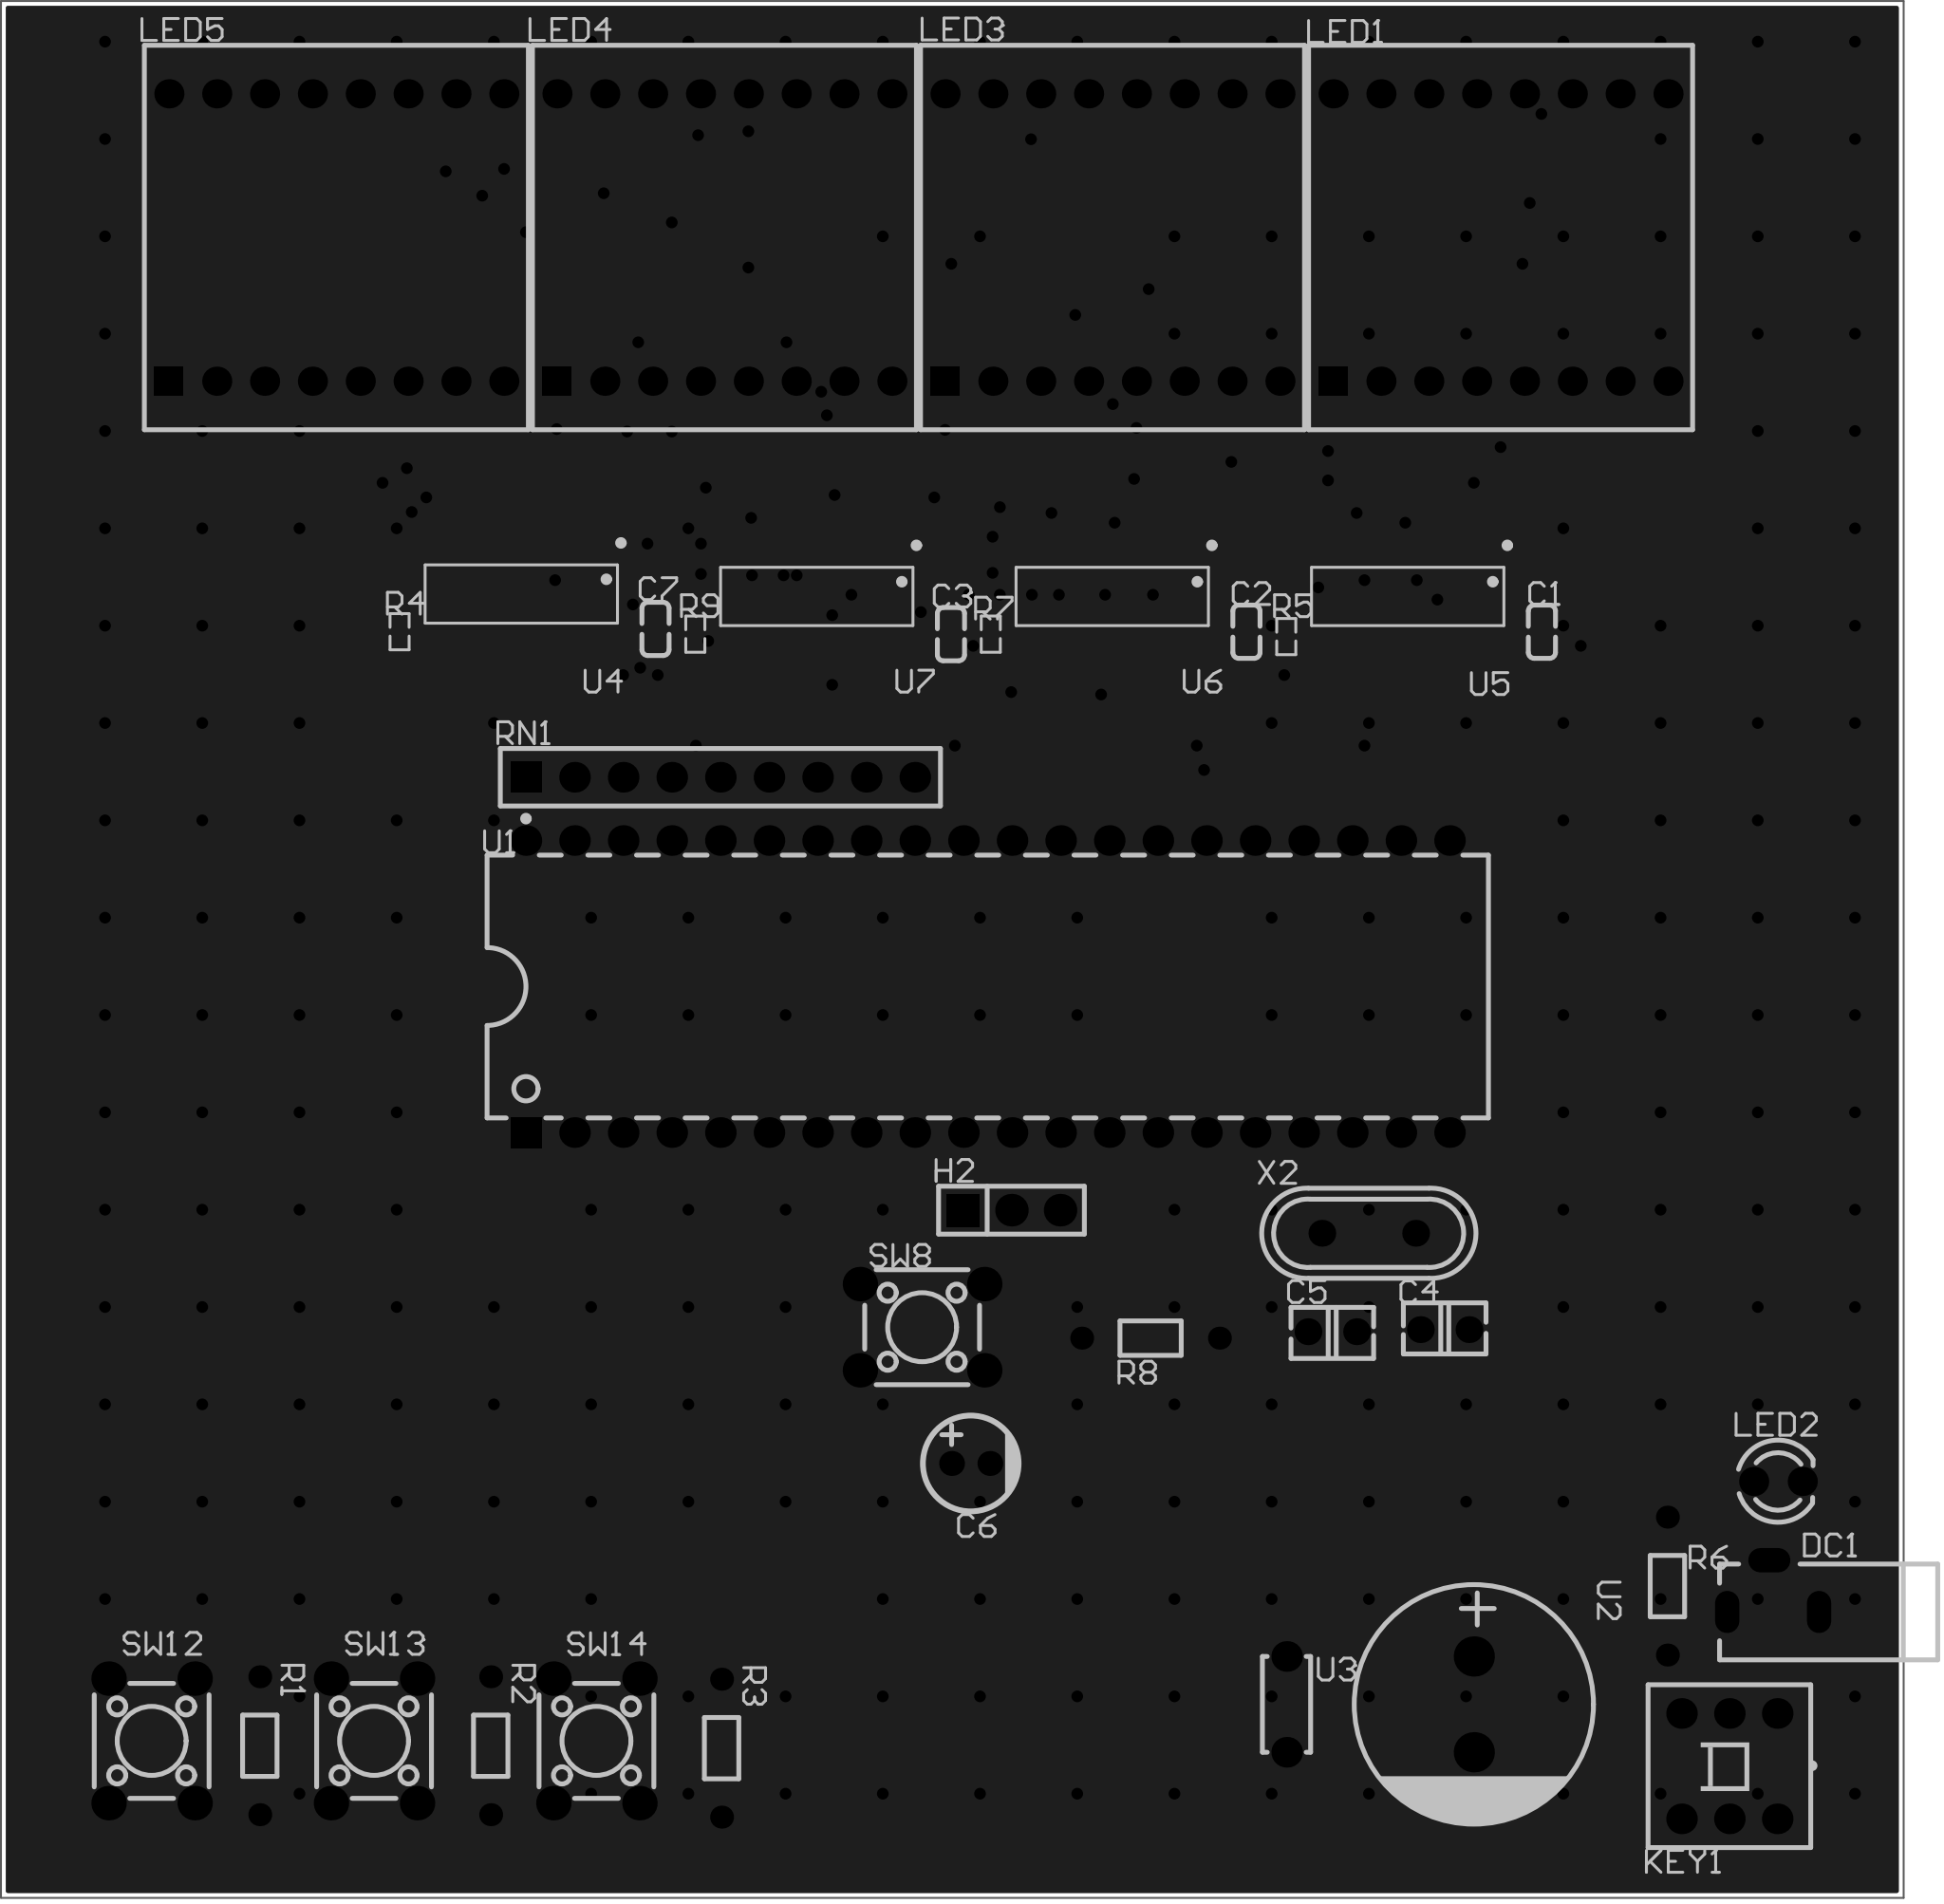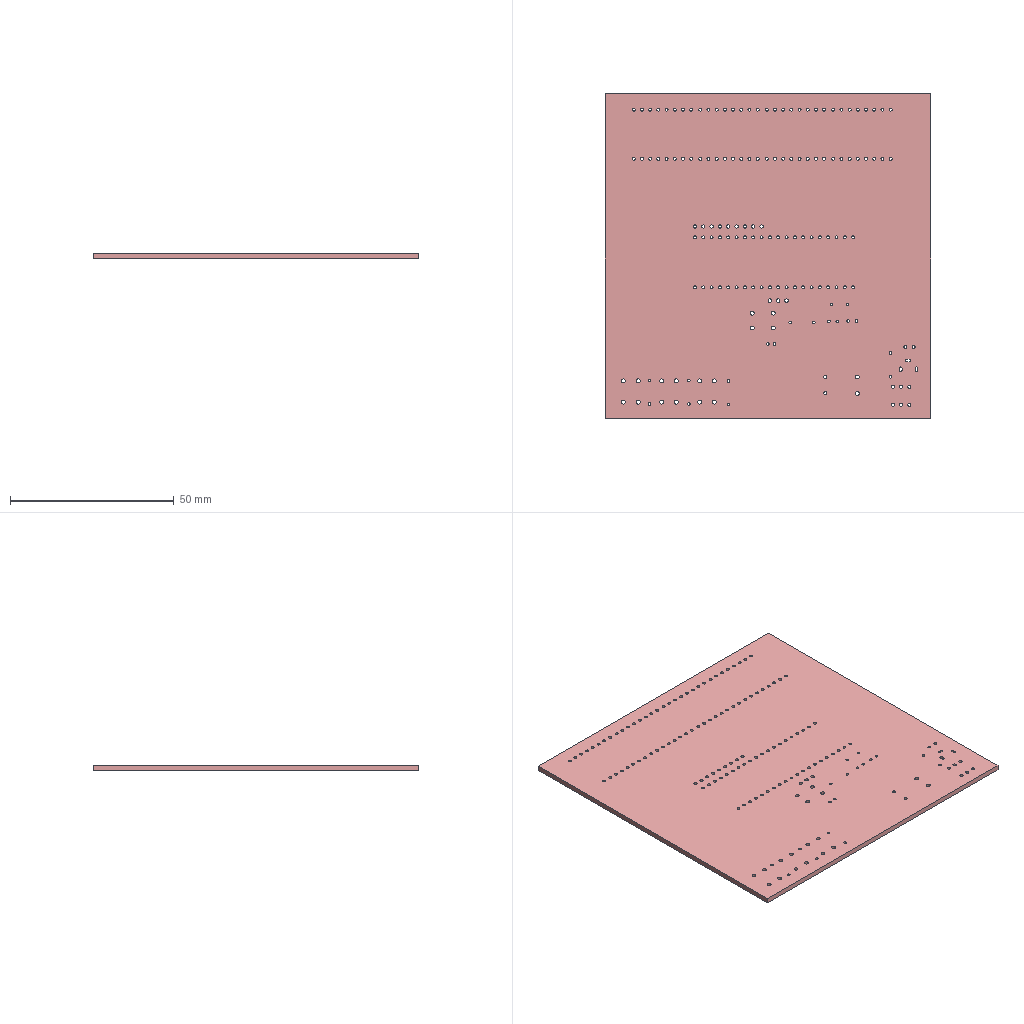Circuit board layout | Altium Designer | box 99.4 x 99 x 1.6 mm
Layer stack:
# Altium Designer layer stack of  (unit mm; dielectric type: 0 none, 1 core, 2 prepreg, 3 surface material)
index,name,kind,layer,copper_thickness_mm,dielectric_type,dielectric_thickness_mm,dielectric_material,dielectric_constant
0,Top Paste Mask Layer,other,,,,,,
1,Top Silkscreen Layer,other,,,,,,
2,Top Solder Mask Layer,dielectric,,,3,0.01,,3.3
3,Top Layer,copper,Top Layer,0.035,,,,
4,Dielectric1,dielectric,,,3,1.51,FR4,4.5
5,Bottom Layer,copper,Bottom Layer,0.035,,,,
6,Bottom Solder Mask Layer,dielectric,,,3,0.01,,3.3
7,Bottom Silkscreen Layer,other,,,,,,
8,Bottom Paste Mask Layer,other,,,,,,
# drill layer pairs: low layer,high layer
drill_pair,Top Layer,Bottom Layer
Part placement:
Designator,Comment,Layer,Footprint,Center-X(mm),Center-Y(mm),Rotation
C4,22pF,TopLayer,CAP-TH_L3.8-W2.5-P2.54-D0.50,157.988,115.57,180
C5,22pF,TopLayer,CAP-TH_L3.8-W2.5-P2.54-D0.50,152.116,115.461,0
C6,10uF,TopLayer,CAP-TH_BD5.0-P2.00-D0.8-FD-10UF50VC110GL,133.223,108.585,0
H2,,TopLayer,HDR-TH_3P-P2.54-V-M,135.352,121.805,0
KEY1,Non-latching switch 8.5×8.5 silent,TopLayer,SW-TH_6P-L8.5-W8.5-P2.54,172.865,92.787,180
LED2,,TopLayer,LED_TH-3mm,175.405,107.646,0
R8,10kΩ,TopLayer,Res_1/8W,142.621,115.126,180
R6,1kΩ,TopLayer,Res_1/8W,169.626,102.185,270
SW8,,TopLayer,SW-TH_4P-L6.0-W6.0-P4.50-LS6.5,130.683,115.697,0
SW12,,TopLayer,SW-TH_4P-L6.0-W6.0-P4.50-LS6.5,90.424,94.107,270
SW13,,TopLayer,SW-TH_4P-L6.0-W6.0-P4.50-LS6.5,102.044,94.107,270
SW14,,TopLayer,SW-TH_4P-L6.0-W6.0-P4.50-LS6.5,113.665,94.107,270
U1,STC89C52RC-40I-PDIP40,TopLayer,DIP-40_L52.0-W13.7-P2.54-LS15.2-BL,134.112,133.477,0
X2,11.059MHz,TopLayer,OSC-TH_L11.1-W4.7-P4.88,154.021,120.6,0
DC1,DC-002,TopLayer,DC-IN-TH_DC-3510,175.151,102.185,0
R1,10kΩ,TopLayer,Res_1/8W,96.075,93.853,270
R2,10kΩ,TopLayer,Res_1/8W,108.14,93.853,270
R3,10kΩ,TopLayer,Res_1/8W,120.205,93.726,270
RN1,-,TopLayer,RES-ARRAY-TH_9P-P2.54-D1.0,120.142,144.399,0
U2,1000uF,TopLayer,CAP-TH_BD12.5-P5.00-D0.6-FD,159.512,96.012,270
U3,100nF,TopLayer,CAP-TH_L5.0-W2.5-P5.00-D1.0,149.733,96.012,270
C1,100nF,TopLayer,C0603,163.068,151.995,270
C2,100nF,TopLayer,C0603,147.629,151.995,270
C3,100nF,TopLayer,C0603,132.19,151.868,270
C7,100nF,TopLayer,C0603,116.751,152.141,270
R4,10kΩ,TopLayer,R0402,103.378,151.995,270
R5,10kΩ,TopLayer,R0402,149.709,151.741,270
R7,10kΩ,TopLayer,R0402,134.27,151.868,270
R9,10kΩ,TopLayer,R0402,118.831,151.868,270
U4,74HC595D,118,TopLayer,SOIC-16_L9.9-W3.9-P1.27-LS6.0-BL,109.738,153.962,180
U5,74HC595D,118,TopLayer,SOIC-16_L9.9-W3.9-P1.27-LS6.0-BL,156.055,153.835,180
U6,74HC595D,118,TopLayer,SOIC-16_L9.9-W3.9-P1.27-LS6.0-BL,140.616,153.835,180
U7,74HC595D,118,TopLayer,SOIC-16_L9.9-W3.9-P1.27-LS6.0-BL,125.177,153.835,180
LED3,SLD0888FR1C1BD-3.5D,TopLayer,LED-MAT-TH_SLD0888FR1C1BD-3.5D,140.631,172.569,0
LED4,SLD0888FR1C1BD-3.5D,TopLayer,LED-MAT-TH_SLD0888FR1C1BD-3.5D,120.354,172.569,0
LED1,SLD0888FR1C1BD-3.5D,TopLayer,LED-MAT-TH_SLD0888FR1C1BD-3.5D,160.909,172.569,0
LED5,SLD0888FR1C1BD-3.5D,TopLayer,LED-MAT-TH_SLD0888FR1C1BD-3.5D,100.076,172.569,0
Pad and via stacks:
# Altium Designer via and pad stacks of  (unit mm). Each distinct definition once, with the count of objects using it.
# via: kind,start_layer,end_layer,hole_mm,diameter_mm,mode(0 simple;1 top-mid-bottom;2 full stack),diameter_per_layer,count,example_net
# pad: kind,layer,hole_mm,hole_type(0 round;1 square;2 slot),plating,top_size,top_shape(1 round;2 rect;3 octagon;9 rounded rect),mid_size,bottom_size,mode,footprint,size_per_layer,count,example
pad,Multi-Layer,0.8,0,plated,1.4x1.4,1,1.4x1.4,1.4x1.4,0,CAP-TH_L3.8-W2.5-P2.54-D0.50,,4,C4.1
pad,Multi-Layer,0.8,0,plated,1.3x1.3,1,1.3x1.3,1.3x1.3,0,CAP-TH_BD5.0-P2.00-D0.8-FD-10UF50VC110GL,,2,C6.2
pad,Multi-Layer,1.1,0,plated,1.7x1.7,2,1.7x1.7,1.7x1.7,0,HDR-TH_3P-P2.54-V-M,,1,H2.1
pad,Multi-Layer,1.1,0,plated,1.7x1.7,1,1.7x1.7,1.7x1.7,0,HDR-TH_3P-P2.54-V-M,,2,H2.2
pad,Multi-Layer,1,0,plated,1.6x1.6,1,1.6x1.6,1.6x1.6,0,SW-TH_6P-L8.5-W8.5-P2.54,,6,KEY1.4
pad,Multi-Layer,0.9144,0,plated,1.524x1.524,1,1.524x1.524,1.524x1.524,0,LED_TH-3mm,,2,LED2.1
pad,Multi-Layer,0.8001,0,plated,1.199x1.199,1,1.199x1.199,1.199x1.199,0,Res_1/8W,,10,R8.1
pad,Multi-Layer,1.2,0,plated,1.8x1.8,1,1.8x1.8,1.8x1.8,0,SW-TH_4P-L6.0-W6.0-P4.50-LS6.5,,16,SW8.1
pad,Multi-Layer,0.889,0,plated,1.6x1.6,1,1.6x1.6,1.6x1.6,0,DIP-40_L52.0-W13.7-P2.54-LS15.2-BL,,39,U1.31
pad,Multi-Layer,0.889,0,plated,1.6x1.6,2,1.6x1.6,1.6x1.6,0,DIP-40_L52.0-W13.7-P2.54-LS15.2-BL,,1,U1.1
pad,Multi-Layer,0.7,0,plated,1.4x1.4,1,1.4x1.4,1.4x1.4,0,OSC-TH_L11.1-W4.7-P4.88,,2,X2.1
pad,Multi-Layer,0.8,2,plated,2.2x1.27,1,2.2x1.27,2.2x1.27,0,DC-IN-TH_DC-3510,,3,DC1.3
pad,Multi-Layer,1,0,plated,1.6x1.6,2,1.6x1.6,1.6x1.6,0,RES-ARRAY-TH_9P-P2.54-D1.0,,1,RN1.1
pad,Multi-Layer,1,0,plated,1.6x1.6,1,1.6x1.6,1.6x1.6,0,RES-ARRAY-TH_9P-P2.54-D1.0,,8,RN1.2
pad,Multi-Layer,1.2,0,plated,2.1x2.1,1,2.1x2.1,2.1x2.1,0,CAP-TH_BD12.5-P5.00-D0.6-FD,,2,U2.1
pad,Multi-Layer,1,0,plated,1.6x1.6,1,1.6x1.6,1.6x1.6,0,CAP-TH_L5.0-W2.5-P5.00-D1.0,,2,U3.1
pad,Multi-Layer,0.9144,0,plated,1.524x1.524,2,1.524x1.524,1.524x1.524,0,LED-MAT-TH_SLD0888FR1C1BD-3.5D,,4,LED3.1
pad,Multi-Layer,0.9144,0,plated,1.524x1.524,1,1.524x1.524,1.524x1.524,0,LED-MAT-TH_SLD0888FR1C1BD-3.5D,,60,LED3.2
pad,Top Layer,0,0,plated,0.8x0.9,2,0.8x0.9,0.8x0.9,0,C0603,,8,C1.2
pad,Top Layer,0,0,plated,0.5657x0.54,2,0.5657x0.54,0.5657x0.54,0,R0402,,8,R4.2
pad,Top Layer,0,0,plated,0.602x1.971,1,0.602x1.971,0.602x1.971,0,SOIC-16_L9.9-W3.9-P1.27-LS6.0-BL,,64,U4.1
via,Top Layer,Bottom Layer,0.3048,0.61,0,,321,A15
Copper pours:
name,layer,net,type(0 solid;1 hatched;2 none)
Top Layer-GND,Top Layer,GND,0
Bottom Layer-GND,Bottom Layer,GND,0
Design rules, without the lines most boards share:
# Altium Designer design rules of  (exported by Altium Designer, unit mm)
# columns: name | kind | enabled | priority | scope1 | scope2 | descriptor | typed fields (field=value)
creepage | 65 | enabled | 1 | All | All | Creepage Distance Constraint =(0mil) (All),(All) |